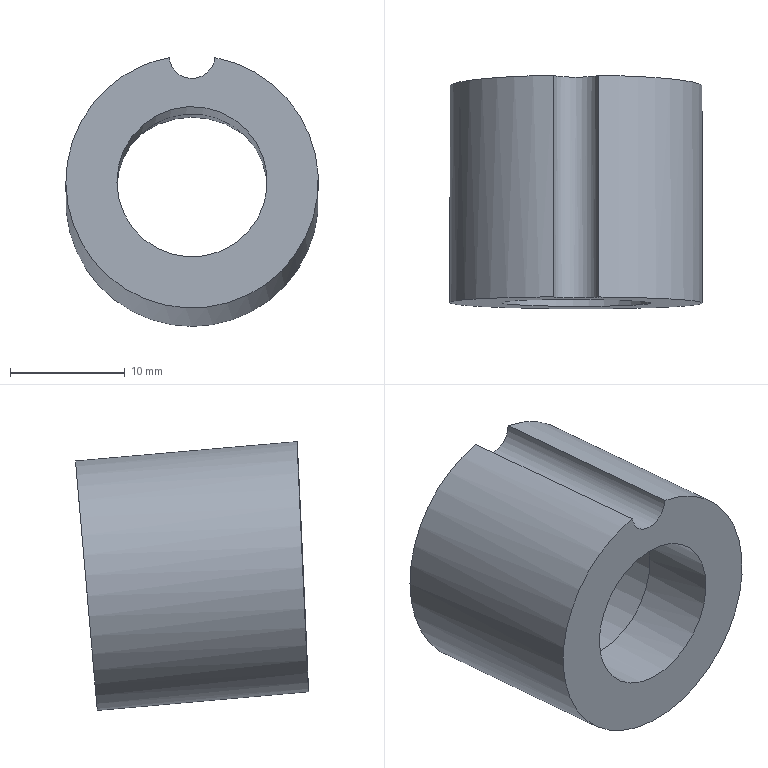Part | NX | features EKSD 22-20-13.10 2 | 1 solid | 7 faces | box 22 x 20.309 x 23.425 mm | volume 4138 mm3 | cylinder 4 | plane 3 | commonest cylinder face diameters 4 x1 13.1 x1 14.6 x1 22 x1
STEP:
#1=CARTESIAN_POINT('',(116.945,-26.467,-29.21));
#2=VERTEX_POINT('',#1);
#3=CARTESIAN_POINT('',(120.928,-26.467,-29.21));
#4=VERTEX_POINT('',#3);
#5=CARTESIAN_POINT('',(118.936,-26.451,-29.029));
#6=DIRECTION('',(0.,-0.9962,0.08716));
#7=DIRECTION('',(0.,-0.08716,-0.9962));
#8=AXIS2_PLACEMENT_3D('',#5,#6,#7);
#9=CIRCLE('',#8,2.);
#10=EDGE_CURVE('',#2,#4,#9,.T.);
#11=ORIENTED_EDGE('',*,*,#10,.T.);
#12=CARTESIAN_POINT('',(118.936,-27.41,-39.987));
#13=DIRECTION('',(0.,-0.9962,0.08716));
#14=DIRECTION('',(0.,-0.08716,-0.9962));
#15=AXIS2_PLACEMENT_3D('',#12,#13,#14);
#16=CIRCLE('',#15,11.);
#17=EDGE_CURVE('',#2,#4,#16,.T.);
#18=ORIENTED_EDGE('',*,*,#17,.F.);
#19=EDGE_LOOP('',(#11,#18));
#20=FACE_BOUND('',#19,.T.);
#21=CARTESIAN_POINT('',(118.936,-26.773,-32.715));
#22=VERTEX_POINT('',#21);
#23=CARTESIAN_POINT('',(118.936,-27.41,-39.987));
#24=DIRECTION('',(0.,0.9962,-0.08716));
#25=DIRECTION('',(0.,0.08716,0.9962));
#26=AXIS2_PLACEMENT_3D('',#23,#24,#25);
#27=CIRCLE('',#26,7.3);
#28=EDGE_CURVE('',#22,#22,#27,.T.);
#29=ORIENTED_EDGE('',*,*,#28,.F.);
#30=EDGE_LOOP('',(#29));
#31=FACE_BOUND('',#30,.T.);
#32=CARTESIAN_POINT('',(118.936,-27.41,-39.987));
#33=DIRECTION('',(0.,0.9962,-0.08716));
#34=DIRECTION('',(0.,0.08716,0.9962));
#35=AXIS2_PLACEMENT_3D('',#32,#33,#34);
#36=PLANE('',#35);
#37=ADVANCED_FACE('',(#20,#31),#36,.T.);
#38=CARTESIAN_POINT('',(120.928,-45.786,-27.52));
#39=VERTEX_POINT('',#38);
#40=CARTESIAN_POINT('',(116.945,-45.779,-27.521));
#41=VERTEX_POINT('',#40);
#42=CARTESIAN_POINT('',(118.936,-45.774,-27.338));
#43=DIRECTION('',(0.001957,0.999,-0.04546));
#44=DIRECTION('',(-0.04675,-0.04532,-0.9979));
#45=AXIS2_PLACEMENT_3D('',#42,#43,#44);
#46=ELLIPSE('',#45,2.002,2.);
#47=EDGE_CURVE('',#39,#41,#46,.T.);
#48=ORIENTED_EDGE('',*,*,#47,.T.);
#49=CARTESIAN_POINT('',(118.936,-46.275,-38.337));
#50=DIRECTION('',(0.001957,0.999,-0.04546));
#51=DIRECTION('',(-0.04675,-0.04532,-0.9979));
#52=AXIS2_PLACEMENT_3D('',#49,#50,#51);
#53=ELLIPSE('',#52,11.01,11.);
#54=EDGE_CURVE('',#39,#41,#53,.T.);
#55=ORIENTED_EDGE('',*,*,#54,.F.);
#56=EDGE_LOOP('',(#48,#55));
#57=FACE_BOUND('',#56,.T.);
#58=CARTESIAN_POINT('',(118.63,-46.572,-44.878));
#59=VERTEX_POINT('',#58);
#60=CARTESIAN_POINT('',(118.936,-46.275,-38.337));
#61=DIRECTION('',(0.001957,0.999,-0.04546));
#62=DIRECTION('',(-0.04675,-0.04532,-0.9979));
#63=AXIS2_PLACEMENT_3D('',#60,#61,#62);
#64=ELLIPSE('',#63,6.556,6.55);
#65=EDGE_CURVE('',#59,#59,#64,.F.);
#66=ORIENTED_EDGE('',*,*,#65,.F.);
#67=EDGE_LOOP('',(#66));
#68=FACE_BOUND('',#67,.T.);
#69=CARTESIAN_POINT('',(128.811,-48.589,-88.763));
#70=DIRECTION('',(0.001957,0.999,-0.04546));
#71=DIRECTION('',(0.06617,0.04523,0.9968));
#72=AXIS2_PLACEMENT_3D('',#69,#70,#71);
#73=PLANE('',#72);
#74=ADVANCED_FACE('',(#57,#68),#73,.F.);
#75=CARTESIAN_POINT('',(120.928,-36.429,-28.339));
#76=DIRECTION('',(0.,0.9962,-0.08716));
#77=VECTOR('',#76,1000.);
#78=LINE('',#75,#77);
#79=EDGE_CURVE('',#39,#4,#78,.T.);
#80=ORIENTED_EDGE('',*,*,#79,.F.);
#81=ORIENTED_EDGE('',*,*,#54,.T.);
#82=CARTESIAN_POINT('',(116.945,-36.429,-28.339));
#83=DIRECTION('',(0.,0.9962,-0.08716));
#84=VECTOR('',#83,1000.);
#85=LINE('',#82,#84);
#86=EDGE_CURVE('',#2,#41,#85,.F.);
#87=ORIENTED_EDGE('',*,*,#86,.F.);
#88=ORIENTED_EDGE('',*,*,#17,.T.);
#89=EDGE_LOOP('',(#80,#81,#87,#88));
#90=FACE_BOUND('',#89,.T.);
#91=CARTESIAN_POINT('',(118.936,-47.333,-38.244));
#92=DIRECTION('',(0.,0.9962,-0.08716));
#93=DIRECTION('',(0.,0.08716,0.9962));
#94=AXIS2_PLACEMENT_3D('',#91,#92,#93);
#95=CYLINDRICAL_SURFACE('',#94,11.);
#96=ADVANCED_FACE('',(#90),#95,.T.);
#97=CARTESIAN_POINT('',(118.936,-39.935,-45.466));
#98=VERTEX_POINT('',#97);
#99=CARTESIAN_POINT('',(118.936,-39.364,-38.941));
#100=DIRECTION('',(0.,-0.9962,0.08716));
#101=DIRECTION('',(0.,-0.08716,-0.9962));
#102=AXIS2_PLACEMENT_3D('',#99,#100,#101);
#103=CIRCLE('',#102,6.55);
#104=EDGE_CURVE('',#98,#98,#103,.F.);
#105=ORIENTED_EDGE('',*,*,#104,.T.);
#106=EDGE_LOOP('',(#105));
#107=FACE_BOUND('',#106,.T.);
#108=ORIENTED_EDGE('',*,*,#65,.T.);
#109=EDGE_LOOP('',(#108));
#110=FACE_BOUND('',#109,.T.);
#111=CARTESIAN_POINT('',(118.936,-48.33,-38.157));
#112=DIRECTION('',(0.,0.9962,-0.08716));
#113=DIRECTION('',(0.,0.08716,0.9962));
#114=AXIS2_PLACEMENT_3D('',#111,#112,#113);
#115=CYLINDRICAL_SURFACE('',#114,6.55);
#116=ADVANCED_FACE('',(#107,#110),#115,.F.);
#117=CARTESIAN_POINT('',(118.936,-38.728,-31.669));
#118=VERTEX_POINT('',#117);
#119=CARTESIAN_POINT('',(118.936,-39.364,-38.941));
#120=DIRECTION('',(0.,0.9962,-0.08716));
#121=DIRECTION('',(0.,0.08716,0.9962));
#122=AXIS2_PLACEMENT_3D('',#119,#120,#121);
#123=CIRCLE('',#122,7.3);
#124=EDGE_CURVE('',#118,#118,#123,.T.);
#125=ORIENTED_EDGE('',*,*,#124,.T.);
#126=EDGE_LOOP('',(#125));
#127=FACE_BOUND('',#126,.T.);
#128=ORIENTED_EDGE('',*,*,#104,.F.);
#129=EDGE_LOOP('',(#128));
#130=FACE_BOUND('',#129,.T.);
#131=CARTESIAN_POINT('',(118.936,-39.364,-38.941));
#132=DIRECTION('',(0.,-0.9962,0.08716));
#133=DIRECTION('',(0.,-0.08716,-0.9962));
#134=AXIS2_PLACEMENT_3D('',#131,#132,#133);
#135=PLANE('',#134);
#136=ADVANCED_FACE('',(#127,#130),#135,.F.);
#137=ORIENTED_EDGE('',*,*,#28,.T.);
#138=EDGE_LOOP('',(#137));
#139=FACE_BOUND('',#138,.T.);
#140=ORIENTED_EDGE('',*,*,#124,.F.);
#141=EDGE_LOOP('',(#140));
#142=FACE_BOUND('',#141,.T.);
#143=CARTESIAN_POINT('',(118.936,-39.364,-38.941));
#144=DIRECTION('',(0.,0.9962,-0.08716));
#145=DIRECTION('',(0.,0.08716,0.9962));
#146=AXIS2_PLACEMENT_3D('',#143,#144,#145);
#147=CYLINDRICAL_SURFACE('',#146,7.3);
#148=ADVANCED_FACE('',(#139,#142),#147,.F.);
#149=ORIENTED_EDGE('',*,*,#79,.T.);
#150=ORIENTED_EDGE('',*,*,#10,.F.);
#151=ORIENTED_EDGE('',*,*,#86,.T.);
#152=ORIENTED_EDGE('',*,*,#47,.F.);
#153=EDGE_LOOP('',(#149,#150,#151,#152));
#154=FACE_BOUND('',#153,.T.);
#155=CARTESIAN_POINT('',(118.936,-46.375,-27.286));
#156=DIRECTION('',(0.,0.9962,-0.08716));
#157=DIRECTION('',(0.,0.08716,0.9962));
#158=AXIS2_PLACEMENT_3D('',#155,#156,#157);
#159=CYLINDRICAL_SURFACE('',#158,2.);
#160=ADVANCED_FACE('',(#154),#159,.F.);
#161=CLOSED_SHELL('',(#37,#74,#96,#116,#136,#148,#160));
#162=MANIFOLD_SOLID_BREP('',#161);
#163=(LENGTH_UNIT()NAMED_UNIT(*)SI_UNIT(.MILLI.,.METRE.));
#164=UNCERTAINTY_MEASURE_WITH_UNIT(LENGTH_MEASURE(0.00001),#163,'','');
#165=(NAMED_UNIT(*)PLANE_ANGLE_UNIT()SI_UNIT($,.RADIAN.));
#166=(NAMED_UNIT(*)SI_UNIT($,.STERADIAN.)SOLID_ANGLE_UNIT());
#167=(GEOMETRIC_REPRESENTATION_CONTEXT(3)GLOBAL_UNCERTAINTY_ASSIGNED_CONTEXT((#164))GLOBAL_UNIT_ASSIGNED_CONTEXT((#163,#165,#166))REPRESENTATION_CONTEXT('',''));
#168=ADVANCED_BREP_SHAPE_REPRESENTATION('',(#162),#167);